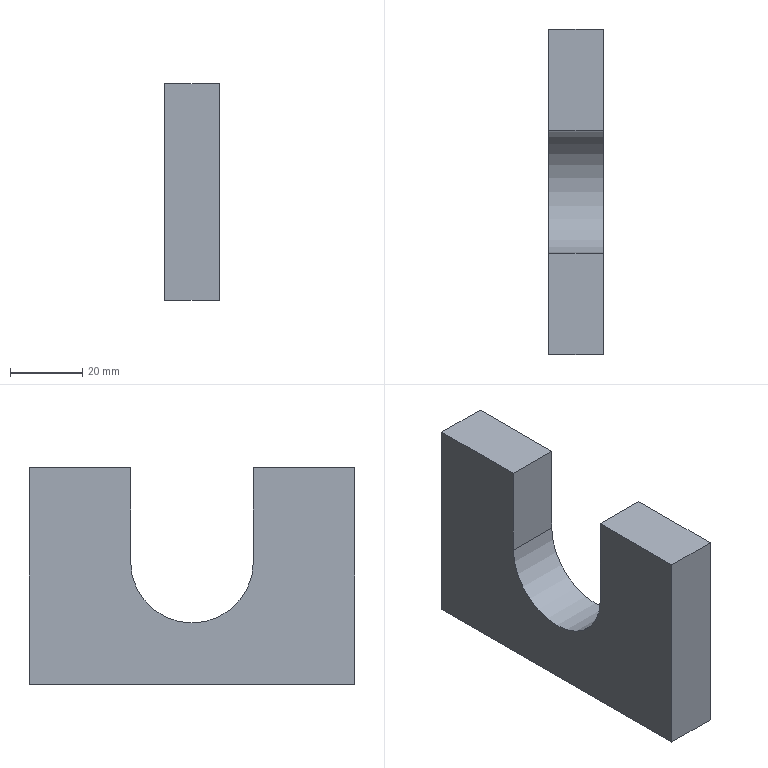Part | STEP file | Tube necking machine_id570_x_t | 1 solid | 10 faces | box 15 x 90 x 60 mm | volume 60931 mm3 | plane 9 | cylinder 1 | commonest cylinder face diameters 34 x1
STEP:
#1=CARTESIAN_POINT('',(0.,0.,0.));
#2=DIRECTION('',(0.,0.,1.));
#3=DIRECTION('',(1.,0.,0.));
#4=AXIS2_PLACEMENT_3D('',#1,#2,#3);
#5=CARTESIAN_POINT('',(305.5,33.,216.));
#6=VERTEX_POINT('',#5);
#7=CARTESIAN_POINT('',(305.5,33.,190.));
#8=VERTEX_POINT('',#7);
#9=CARTESIAN_POINT('',(305.5,33.,252.));
#10=DIRECTION('',(0.,0.,-1.));
#11=VECTOR('',#10,1.);
#12=LINE('',#9,#11);
#13=CARTESIAN_POINT('',(305.5,5.,252.));
#14=DIRECTION('',(-1.,0.,0.));
#15=DIRECTION('',(0.,0.,1.));
#16=AXIS2_PLACEMENT_3D('',#13,#14,#15);
#17=PLANE('',#16);
#18=CARTESIAN_POINT('',(0.,28.));
#19=DIRECTION('',(-1.,0.));
#20=VECTOR('',#19,1.);
#21=LINE('',#18,#20);
#22=(GEOMETRIC_REPRESENTATION_CONTEXT(2)PARAMETRIC_REPRESENTATION_CONTEXT()REPRESENTATION_CONTEXT('',''));
#23=DEFINITIONAL_REPRESENTATION('',(#21),#22);
#24=PCURVE('',#17,#23);
#25=CARTESIAN_POINT('',(320.5,33.,231.));
#26=DIRECTION('',(0.,1.,0.));
#27=DIRECTION('',(0.,0.,1.));
#28=AXIS2_PLACEMENT_3D('',#25,#26,#27);
#29=PLANE('',#28);
#30=CARTESIAN_POINT('',(21.,-15.));
#31=DIRECTION('',(-1.,0.));
#32=VECTOR('',#31,1.);
#33=LINE('',#30,#32);
#34=(GEOMETRIC_REPRESENTATION_CONTEXT(2)PARAMETRIC_REPRESENTATION_CONTEXT()REPRESENTATION_CONTEXT('',''));
#35=DEFINITIONAL_REPRESENTATION('',(#33),#34);
#36=PCURVE('',#29,#35);
#37=SURFACE_CURVE('',#12,(#24,#36),.PCURVE_S1.);
#38=EDGE_CURVE('',#6,#8,#37,.T.);
#39=ORIENTED_EDGE('',*,*,#38,.F.);
#40=CARTESIAN_POINT('',(305.5,5.,216.));
#41=VERTEX_POINT('',#40);
#42=CARTESIAN_POINT('',(305.5,5.,216.));
#43=DIRECTION('',(0.,1.,0.));
#44=VECTOR('',#43,1.);
#45=LINE('',#42,#44);
#46=CARTESIAN_POINT('',(-36.,0.));
#47=DIRECTION('',(0.,1.));
#48=VECTOR('',#47,1.);
#49=LINE('',#46,#48);
#50=(GEOMETRIC_REPRESENTATION_CONTEXT(2)PARAMETRIC_REPRESENTATION_CONTEXT()REPRESENTATION_CONTEXT('',''));
#51=DEFINITIONAL_REPRESENTATION('',(#49),#50);
#52=PCURVE('',#17,#51);
#53=CARTESIAN_POINT('',(8.,0.,216.));
#54=DIRECTION('',(0.,0.,1.));
#55=DIRECTION('',(1.,0.,0.));
#56=AXIS2_PLACEMENT_3D('',#53,#54,#55);
#57=PLANE('',#56);
#58=CARTESIAN_POINT('',(297.5,5.));
#59=DIRECTION('',(0.,1.));
#60=VECTOR('',#59,1.);
#61=LINE('',#58,#60);
#62=(GEOMETRIC_REPRESENTATION_CONTEXT(2)PARAMETRIC_REPRESENTATION_CONTEXT()REPRESENTATION_CONTEXT('',''));
#63=DEFINITIONAL_REPRESENTATION('',(#61),#62);
#64=PCURVE('',#57,#63);
#65=SURFACE_CURVE('',#45,(#52,#64),.PCURVE_S1.);
#66=EDGE_CURVE('',#41,#6,#65,.T.);
#67=ORIENTED_EDGE('',*,*,#66,.F.);
#68=CARTESIAN_POINT('',(305.5,5.,156.));
#69=VERTEX_POINT('',#68);
#70=CARTESIAN_POINT('',(305.5,5.,252.));
#71=DIRECTION('',(0.,0.,-1.));
#72=VECTOR('',#71,1.);
#73=LINE('',#70,#72);
#74=CARTESIAN_POINT('',(0.,0.));
#75=DIRECTION('',(-1.,0.));
#76=VECTOR('',#75,1.);
#77=LINE('',#74,#76);
#78=(GEOMETRIC_REPRESENTATION_CONTEXT(2)PARAMETRIC_REPRESENTATION_CONTEXT()REPRESENTATION_CONTEXT('',''));
#79=DEFINITIONAL_REPRESENTATION('',(#77),#78);
#80=PCURVE('',#17,#79);
#81=CARTESIAN_POINT('',(235.5,5.,252.));
#82=DIRECTION('',(0.,1.,0.));
#83=DIRECTION('',(0.,0.,1.));
#84=AXIS2_PLACEMENT_3D('',#81,#82,#83);
#85=PLANE('',#84);
#86=CARTESIAN_POINT('',(0.,70.));
#87=DIRECTION('',(-1.,0.));
#88=VECTOR('',#87,1.);
#89=LINE('',#86,#88);
#90=(GEOMETRIC_REPRESENTATION_CONTEXT(2)PARAMETRIC_REPRESENTATION_CONTEXT()REPRESENTATION_CONTEXT('',''));
#91=DEFINITIONAL_REPRESENTATION('',(#89),#90);
#92=PCURVE('',#85,#91);
#93=SURFACE_CURVE('',#73,(#80,#92),.PCURVE_S1.);
#94=EDGE_CURVE('',#41,#69,#93,.T.);
#95=ORIENTED_EDGE('',*,*,#94,.T.);
#96=CARTESIAN_POINT('',(305.5,95.,156.));
#97=VERTEX_POINT('',#96);
#98=CARTESIAN_POINT('',(305.5,5.,156.));
#99=DIRECTION('',(0.,1.,0.));
#100=VECTOR('',#99,1.);
#101=LINE('',#98,#100);
#102=CARTESIAN_POINT('',(-96.,0.));
#103=DIRECTION('',(0.,1.));
#104=VECTOR('',#103,1.);
#105=LINE('',#102,#104);
#106=(GEOMETRIC_REPRESENTATION_CONTEXT(2)PARAMETRIC_REPRESENTATION_CONTEXT()REPRESENTATION_CONTEXT('',''));
#107=DEFINITIONAL_REPRESENTATION('',(#105),#106);
#108=PCURVE('',#17,#107);
#109=CARTESIAN_POINT('',(8.,0.,156.));
#110=DIRECTION('',(0.,0.,1.));
#111=DIRECTION('',(1.,0.,0.));
#112=AXIS2_PLACEMENT_3D('',#109,#110,#111);
#113=PLANE('',#112);
#114=CARTESIAN_POINT('',(297.5,5.));
#115=DIRECTION('',(0.,1.));
#116=VECTOR('',#115,1.);
#117=LINE('',#114,#116);
#118=(GEOMETRIC_REPRESENTATION_CONTEXT(2)PARAMETRIC_REPRESENTATION_CONTEXT()REPRESENTATION_CONTEXT('',''));
#119=DEFINITIONAL_REPRESENTATION('',(#117),#118);
#120=PCURVE('',#113,#119);
#121=SURFACE_CURVE('',#101,(#108,#120),.PCURVE_S1.);
#122=EDGE_CURVE('',#69,#97,#121,.T.);
#123=ORIENTED_EDGE('',*,*,#122,.T.);
#124=CARTESIAN_POINT('',(305.5,95.,216.));
#125=VERTEX_POINT('',#124);
#126=CARTESIAN_POINT('',(305.5,95.,252.));
#127=DIRECTION('',(0.,0.,-1.));
#128=VECTOR('',#127,1.);
#129=LINE('',#126,#128);
#130=CARTESIAN_POINT('',(0.,90.));
#131=DIRECTION('',(-1.,0.));
#132=VECTOR('',#131,1.);
#133=LINE('',#130,#132);
#134=(GEOMETRIC_REPRESENTATION_CONTEXT(2)PARAMETRIC_REPRESENTATION_CONTEXT()REPRESENTATION_CONTEXT('',''));
#135=DEFINITIONAL_REPRESENTATION('',(#133),#134);
#136=PCURVE('',#17,#135);
#137=CARTESIAN_POINT('',(305.5,95.,252.));
#138=DIRECTION('',(0.,-1.,0.));
#139=DIRECTION('',(0.,0.,-1.));
#140=AXIS2_PLACEMENT_3D('',#137,#138,#139);
#141=PLANE('',#140);
#142=CARTESIAN_POINT('',(0.,0.));
#143=DIRECTION('',(1.,0.));
#144=VECTOR('',#143,1.);
#145=LINE('',#142,#144);
#146=(GEOMETRIC_REPRESENTATION_CONTEXT(2)PARAMETRIC_REPRESENTATION_CONTEXT()REPRESENTATION_CONTEXT('',''));
#147=DEFINITIONAL_REPRESENTATION('',(#145),#146);
#148=PCURVE('',#141,#147);
#149=SURFACE_CURVE('',#129,(#136,#148),.PCURVE_S1.);
#150=EDGE_CURVE('',#125,#97,#149,.T.);
#151=ORIENTED_EDGE('',*,*,#150,.F.);
#152=CARTESIAN_POINT('',(305.5,67.,216.));
#153=VERTEX_POINT('',#152);
#154=CARTESIAN_POINT('',(305.5,5.,216.));
#155=DIRECTION('',(0.,1.,0.));
#156=VECTOR('',#155,1.);
#157=LINE('',#154,#156);
#158=CARTESIAN_POINT('',(-36.,0.));
#159=DIRECTION('',(0.,1.));
#160=VECTOR('',#159,1.);
#161=LINE('',#158,#160);
#162=(GEOMETRIC_REPRESENTATION_CONTEXT(2)PARAMETRIC_REPRESENTATION_CONTEXT()REPRESENTATION_CONTEXT('',''));
#163=DEFINITIONAL_REPRESENTATION('',(#161),#162);
#164=PCURVE('',#17,#163);
#165=CARTESIAN_POINT('',(8.,0.,216.));
#166=DIRECTION('',(0.,0.,1.));
#167=DIRECTION('',(1.,0.,0.));
#168=AXIS2_PLACEMENT_3D('',#165,#166,#167);
#169=PLANE('',#168);
#170=CARTESIAN_POINT('',(297.5,5.));
#171=DIRECTION('',(0.,1.));
#172=VECTOR('',#171,1.);
#173=LINE('',#170,#172);
#174=(GEOMETRIC_REPRESENTATION_CONTEXT(2)PARAMETRIC_REPRESENTATION_CONTEXT()REPRESENTATION_CONTEXT('',''));
#175=DEFINITIONAL_REPRESENTATION('',(#173),#174);
#176=PCURVE('',#169,#175);
#177=SURFACE_CURVE('',#157,(#164,#176),.PCURVE_S1.);
#178=EDGE_CURVE('',#153,#125,#177,.T.);
#179=ORIENTED_EDGE('',*,*,#178,.F.);
#180=CARTESIAN_POINT('',(305.5,67.,190.));
#181=VERTEX_POINT('',#180);
#182=CARTESIAN_POINT('',(305.5,67.,252.));
#183=DIRECTION('',(0.,0.,1.));
#184=VECTOR('',#183,1.);
#185=LINE('',#182,#184);
#186=CARTESIAN_POINT('',(0.,62.));
#187=DIRECTION('',(1.,0.));
#188=VECTOR('',#187,1.);
#189=LINE('',#186,#188);
#190=(GEOMETRIC_REPRESENTATION_CONTEXT(2)PARAMETRIC_REPRESENTATION_CONTEXT()REPRESENTATION_CONTEXT('',''));
#191=DEFINITIONAL_REPRESENTATION('',(#189),#190);
#192=PCURVE('',#17,#191);
#193=CARTESIAN_POINT('',(320.5,67.,190.));
#194=DIRECTION('',(0.,-1.,0.));
#195=DIRECTION('',(0.,0.,-1.));
#196=AXIS2_PLACEMENT_3D('',#193,#194,#195);
#197=PLANE('',#196);
#198=CARTESIAN_POINT('',(-62.,-15.));
#199=DIRECTION('',(-1.,0.));
#200=VECTOR('',#199,1.);
#201=LINE('',#198,#200);
#202=(GEOMETRIC_REPRESENTATION_CONTEXT(2)PARAMETRIC_REPRESENTATION_CONTEXT()REPRESENTATION_CONTEXT('',''));
#203=DEFINITIONAL_REPRESENTATION('',(#201),#202);
#204=PCURVE('',#197,#203);
#205=SURFACE_CURVE('',#185,(#192,#204),.PCURVE_S1.);
#206=EDGE_CURVE('',#181,#153,#205,.T.);
#207=ORIENTED_EDGE('',*,*,#206,.F.);
#208=CARTESIAN_POINT('',(305.5,50.,190.));
#209=DIRECTION('',(1.,0.,0.));
#210=DIRECTION('',(0.,0.,1.));
#211=AXIS2_PLACEMENT_3D('',#208,#209,#210);
#212=CIRCLE('',#211,17.);
#213=CARTESIAN_POINT('',(-45.,45.));
#214=CARTESIAN_POINT('',(-45.,15.555));
#215=CARTESIAN_POINT('',(-70.5,30.278));
#216=CARTESIAN_POINT('',(-96.,45.));
#217=CARTESIAN_POINT('',(-70.5,59.722));
#218=CARTESIAN_POINT('',(-45.,74.445));
#219=CARTESIAN_POINT('',(-45.,45.));
#220=(BOUNDED_CURVE()B_SPLINE_CURVE(2,(#213,#214,#215,#216,#217,#218,#219),.UNSPECIFIED.,.T.,.F.)B_SPLINE_CURVE_WITH_KNOTS((1,2,2,2,2,1),(-2.094,0.,2.094,4.189,6.283,8.378),.UNSPECIFIED.)CURVE()GEOMETRIC_REPRESENTATION_ITEM()RATIONAL_B_SPLINE_CURVE((1.,0.5,1.,0.5,1.,0.5,1.))REPRESENTATION_ITEM(''));
#221=(GEOMETRIC_REPRESENTATION_CONTEXT(2)PARAMETRIC_REPRESENTATION_CONTEXT()REPRESENTATION_CONTEXT('',''));
#222=DEFINITIONAL_REPRESENTATION('',(#220),#221);
#223=PCURVE('',#17,#222);
#224=CARTESIAN_POINT('',(290.5,50.,190.));
#225=DIRECTION('',(1.,0.,0.));
#226=DIRECTION('',(0.,0.,-1.));
#227=AXIS2_PLACEMENT_3D('',#224,#225,#226);
#228=CYLINDRICAL_SURFACE('',#227,17.);
#229=CARTESIAN_POINT('',(3.142,15.));
#230=DIRECTION('',(1.,0.));
#231=VECTOR('',#230,1.);
#232=LINE('',#229,#231);
#233=(GEOMETRIC_REPRESENTATION_CONTEXT(2)PARAMETRIC_REPRESENTATION_CONTEXT()REPRESENTATION_CONTEXT('',''));
#234=DEFINITIONAL_REPRESENTATION('',(#232),#233);
#235=PCURVE('',#228,#234);
#236=SURFACE_CURVE('',#212,(#223,#235),.PCURVE_S1.);
#237=EDGE_CURVE('',#8,#181,#236,.T.);
#238=ORIENTED_EDGE('',*,*,#237,.F.);
#239=EDGE_LOOP('',(#39,#67,#95,#123,#151,#179,#207,#238));
#240=FACE_BOUND('',#239,.T.);
#241=ADVANCED_FACE('',(#240),#17,.F.);
#242=ORIENTED_EDGE('',*,*,#66,.T.);
#243=CARTESIAN_POINT('',(290.5,33.,216.));
#244=VERTEX_POINT('',#243);
#245=CARTESIAN_POINT('',(8.,33.,216.));
#246=DIRECTION('',(-1.,0.,0.));
#247=VECTOR('',#246,1.);
#248=LINE('',#245,#247);
#249=CARTESIAN_POINT('',(0.,33.));
#250=DIRECTION('',(-1.,0.));
#251=VECTOR('',#250,1.);
#252=LINE('',#249,#251);
#253=(GEOMETRIC_REPRESENTATION_CONTEXT(2)PARAMETRIC_REPRESENTATION_CONTEXT()REPRESENTATION_CONTEXT('',''));
#254=DEFINITIONAL_REPRESENTATION('',(#252),#253);
#255=PCURVE('',#57,#254);
#256=CARTESIAN_POINT('',(-15.,-312.5));
#257=DIRECTION('',(0.,-1.));
#258=VECTOR('',#257,1.);
#259=LINE('',#256,#258);
#260=(GEOMETRIC_REPRESENTATION_CONTEXT(2)PARAMETRIC_REPRESENTATION_CONTEXT()REPRESENTATION_CONTEXT('',''));
#261=DEFINITIONAL_REPRESENTATION('',(#259),#260);
#262=PCURVE('',#29,#261);
#263=SURFACE_CURVE('',#248,(#255,#262),.PCURVE_S1.);
#264=EDGE_CURVE('',#6,#244,#263,.T.);
#265=ORIENTED_EDGE('',*,*,#264,.T.);
#266=CARTESIAN_POINT('',(290.5,5.,216.));
#267=VERTEX_POINT('',#266);
#268=CARTESIAN_POINT('',(290.5,0.,216.));
#269=DIRECTION('',(0.,1.,0.));
#270=VECTOR('',#269,1.);
#271=LINE('',#268,#270);
#272=CARTESIAN_POINT('',(282.5,0.));
#273=DIRECTION('',(0.,1.));
#274=VECTOR('',#273,1.);
#275=LINE('',#272,#274);
#276=(GEOMETRIC_REPRESENTATION_CONTEXT(2)PARAMETRIC_REPRESENTATION_CONTEXT()REPRESENTATION_CONTEXT('',''));
#277=DEFINITIONAL_REPRESENTATION('',(#275),#276);
#278=PCURVE('',#57,#277);
#279=CARTESIAN_POINT('',(290.5,20.,332.));
#280=DIRECTION('',(-1.,0.,0.));
#281=DIRECTION('',(0.,0.,1.));
#282=AXIS2_PLACEMENT_3D('',#279,#280,#281);
#283=PLANE('',#282);
#284=CARTESIAN_POINT('',(-116.,-20.));
#285=DIRECTION('',(0.,1.));
#286=VECTOR('',#285,1.);
#287=LINE('',#284,#286);
#288=(GEOMETRIC_REPRESENTATION_CONTEXT(2)PARAMETRIC_REPRESENTATION_CONTEXT()REPRESENTATION_CONTEXT('',''));
#289=DEFINITIONAL_REPRESENTATION('',(#287),#288);
#290=PCURVE('',#283,#289);
#291=SURFACE_CURVE('',#271,(#278,#290),.PCURVE_S1.);
#292=EDGE_CURVE('',#267,#244,#291,.T.);
#293=ORIENTED_EDGE('',*,*,#292,.F.);
#294=CARTESIAN_POINT('',(235.5,5.,216.));
#295=DIRECTION('',(1.,0.,0.));
#296=VECTOR('',#295,1.);
#297=LINE('',#294,#296);
#298=CARTESIAN_POINT('',(227.5,5.));
#299=DIRECTION('',(1.,0.));
#300=VECTOR('',#299,1.);
#301=LINE('',#298,#300);
#302=(GEOMETRIC_REPRESENTATION_CONTEXT(2)PARAMETRIC_REPRESENTATION_CONTEXT()REPRESENTATION_CONTEXT('',''));
#303=DEFINITIONAL_REPRESENTATION('',(#301),#302);
#304=PCURVE('',#57,#303);
#305=CARTESIAN_POINT('',(-36.,0.));
#306=DIRECTION('',(0.,1.));
#307=VECTOR('',#306,1.);
#308=LINE('',#305,#307);
#309=(GEOMETRIC_REPRESENTATION_CONTEXT(2)PARAMETRIC_REPRESENTATION_CONTEXT()REPRESENTATION_CONTEXT('',''));
#310=DEFINITIONAL_REPRESENTATION('',(#308),#309);
#311=PCURVE('',#85,#310);
#312=SURFACE_CURVE('',#297,(#304,#311),.PCURVE_S1.);
#313=EDGE_CURVE('',#267,#41,#312,.T.);
#314=ORIENTED_EDGE('',*,*,#313,.T.);
#315=EDGE_LOOP('',(#242,#265,#293,#314));
#316=FACE_BOUND('',#315,.T.);
#317=ADVANCED_FACE('',(#316),#57,.T.);
#318=CARTESIAN_POINT('',(290.5,67.,216.));
#319=VERTEX_POINT('',#318);
#320=CARTESIAN_POINT('',(290.5,95.,216.));
#321=VERTEX_POINT('',#320);
#322=CARTESIAN_POINT('',(290.5,0.,216.));
#323=DIRECTION('',(0.,1.,0.));
#324=VECTOR('',#323,1.);
#325=LINE('',#322,#324);
#326=CARTESIAN_POINT('',(282.5,0.));
#327=DIRECTION('',(0.,1.));
#328=VECTOR('',#327,1.);
#329=LINE('',#326,#328);
#330=(GEOMETRIC_REPRESENTATION_CONTEXT(2)PARAMETRIC_REPRESENTATION_CONTEXT()REPRESENTATION_CONTEXT('',''));
#331=DEFINITIONAL_REPRESENTATION('',(#329),#330);
#332=PCURVE('',#169,#331);
#333=CARTESIAN_POINT('',(-116.,-20.));
#334=DIRECTION('',(0.,1.));
#335=VECTOR('',#334,1.);
#336=LINE('',#333,#335);
#337=(GEOMETRIC_REPRESENTATION_CONTEXT(2)PARAMETRIC_REPRESENTATION_CONTEXT()REPRESENTATION_CONTEXT('',''));
#338=DEFINITIONAL_REPRESENTATION('',(#336),#337);
#339=PCURVE('',#283,#338);
#340=SURFACE_CURVE('',#325,(#332,#339),.PCURVE_S1.);
#341=EDGE_CURVE('',#319,#321,#340,.T.);
#342=ORIENTED_EDGE('',*,*,#341,.F.);
#343=CARTESIAN_POINT('',(8.,67.,216.));
#344=DIRECTION('',(1.,0.,0.));
#345=VECTOR('',#344,1.);
#346=LINE('',#343,#345);
#347=CARTESIAN_POINT('',(0.,67.));
#348=DIRECTION('',(1.,0.));
#349=VECTOR('',#348,1.);
#350=LINE('',#347,#349);
#351=(GEOMETRIC_REPRESENTATION_CONTEXT(2)PARAMETRIC_REPRESENTATION_CONTEXT()REPRESENTATION_CONTEXT('',''));
#352=DEFINITIONAL_REPRESENTATION('',(#350),#351);
#353=PCURVE('',#169,#352);
#354=CARTESIAN_POINT('',(-26.,-312.5));
#355=DIRECTION('',(0.,1.));
#356=VECTOR('',#355,1.);
#357=LINE('',#354,#356);
#358=(GEOMETRIC_REPRESENTATION_CONTEXT(2)PARAMETRIC_REPRESENTATION_CONTEXT()REPRESENTATION_CONTEXT('',''));
#359=DEFINITIONAL_REPRESENTATION('',(#357),#358);
#360=PCURVE('',#197,#359);
#361=SURFACE_CURVE('',#346,(#353,#360),.PCURVE_S1.);
#362=EDGE_CURVE('',#319,#153,#361,.T.);
#363=ORIENTED_EDGE('',*,*,#362,.T.);
#364=ORIENTED_EDGE('',*,*,#178,.T.);
#365=CARTESIAN_POINT('',(305.5,95.,216.));
#366=DIRECTION('',(-1.,0.,0.));
#367=VECTOR('',#366,1.);
#368=LINE('',#365,#367);
#369=CARTESIAN_POINT('',(297.5,95.));
#370=DIRECTION('',(-1.,0.));
#371=VECTOR('',#370,1.);
#372=LINE('',#369,#371);
#373=(GEOMETRIC_REPRESENTATION_CONTEXT(2)PARAMETRIC_REPRESENTATION_CONTEXT()REPRESENTATION_CONTEXT('',''));
#374=DEFINITIONAL_REPRESENTATION('',(#372),#373);
#375=PCURVE('',#169,#374);
#376=CARTESIAN_POINT('',(36.,0.));
#377=DIRECTION('',(0.,-1.));
#378=VECTOR('',#377,1.);
#379=LINE('',#376,#378);
#380=(GEOMETRIC_REPRESENTATION_CONTEXT(2)PARAMETRIC_REPRESENTATION_CONTEXT()REPRESENTATION_CONTEXT('',''));
#381=DEFINITIONAL_REPRESENTATION('',(#379),#380);
#382=PCURVE('',#141,#381);
#383=SURFACE_CURVE('',#368,(#375,#382),.PCURVE_S1.);
#384=EDGE_CURVE('',#125,#321,#383,.T.);
#385=ORIENTED_EDGE('',*,*,#384,.T.);
#386=EDGE_LOOP('',(#342,#363,#364,#385));
#387=FACE_BOUND('',#386,.T.);
#388=ADVANCED_FACE('',(#387),#169,.T.);
#389=ORIENTED_EDGE('',*,*,#292,.T.);
#390=CARTESIAN_POINT('',(290.5,33.,190.));
#391=VERTEX_POINT('',#390);
#392=CARTESIAN_POINT('',(290.5,33.,332.));
#393=DIRECTION('',(0.,0.,-1.));
#394=VECTOR('',#393,1.);
#395=LINE('',#392,#394);
#396=CARTESIAN_POINT('',(0.,13.));
#397=DIRECTION('',(-1.,0.));
#398=VECTOR('',#397,1.);
#399=LINE('',#396,#398);
#400=(GEOMETRIC_REPRESENTATION_CONTEXT(2)PARAMETRIC_REPRESENTATION_CONTEXT()REPRESENTATION_CONTEXT('',''));
#401=DEFINITIONAL_REPRESENTATION('',(#399),#400);
#402=PCURVE('',#283,#401);
#403=CARTESIAN_POINT('',(101.,-30.));
#404=DIRECTION('',(-1.,0.));
#405=VECTOR('',#404,1.);
#406=LINE('',#403,#405);
#407=(GEOMETRIC_REPRESENTATION_CONTEXT(2)PARAMETRIC_REPRESENTATION_CONTEXT()REPRESENTATION_CONTEXT('',''));
#408=DEFINITIONAL_REPRESENTATION('',(#406),#407);
#409=PCURVE('',#29,#408);
#410=SURFACE_CURVE('',#395,(#402,#409),.PCURVE_S1.);
#411=EDGE_CURVE('',#244,#391,#410,.T.);
#412=ORIENTED_EDGE('',*,*,#411,.T.);
#413=CARTESIAN_POINT('',(290.5,67.,190.));
#414=VERTEX_POINT('',#413);
#415=CARTESIAN_POINT('',(290.5,50.,190.));
#416=DIRECTION('',(1.,0.,0.));
#417=DIRECTION('',(0.,0.,1.));
#418=AXIS2_PLACEMENT_3D('',#415,#416,#417);
#419=CIRCLE('',#418,17.);
#420=CARTESIAN_POINT('',(-125.,30.));
#421=CARTESIAN_POINT('',(-125.,0.5551));
#422=CARTESIAN_POINT('',(-150.5,15.278));
#423=CARTESIAN_POINT('',(-176.,30.));
#424=CARTESIAN_POINT('',(-150.5,44.722));
#425=CARTESIAN_POINT('',(-125.,59.445));
#426=CARTESIAN_POINT('',(-125.,30.));
#427=(BOUNDED_CURVE()B_SPLINE_CURVE(2,(#420,#421,#422,#423,#424,#425,#426),.UNSPECIFIED.,.T.,.F.)B_SPLINE_CURVE_WITH_KNOTS((1,2,2,2,2,1),(-2.094,0.,2.094,4.189,6.283,8.378),.UNSPECIFIED.)CURVE()GEOMETRIC_REPRESENTATION_ITEM()RATIONAL_B_SPLINE_CURVE((1.,0.5,1.,0.5,1.,0.5,1.))REPRESENTATION_ITEM(''));
#428=(GEOMETRIC_REPRESENTATION_CONTEXT(2)PARAMETRIC_REPRESENTATION_CONTEXT()REPRESENTATION_CONTEXT('',''));
#429=DEFINITIONAL_REPRESENTATION('',(#427),#428);
#430=PCURVE('',#283,#429);
#431=CARTESIAN_POINT('',(3.142,0.));
#432=DIRECTION('',(1.,0.));
#433=VECTOR('',#432,1.);
#434=LINE('',#431,#433);
#435=(GEOMETRIC_REPRESENTATION_CONTEXT(2)PARAMETRIC_REPRESENTATION_CONTEXT()REPRESENTATION_CONTEXT('',''));
#436=DEFINITIONAL_REPRESENTATION('',(#434),#435);
#437=PCURVE('',#228,#436);
#438=SURFACE_CURVE('',#419,(#430,#437),.PCURVE_S1.);
#439=EDGE_CURVE('',#391,#414,#438,.T.);
#440=ORIENTED_EDGE('',*,*,#439,.T.);
#441=CARTESIAN_POINT('',(290.5,67.,332.));
#442=DIRECTION('',(0.,0.,1.));
#443=VECTOR('',#442,1.);
#444=LINE('',#441,#443);
#445=CARTESIAN_POINT('',(0.,47.));
#446=DIRECTION('',(1.,0.));
#447=VECTOR('',#446,1.);
#448=LINE('',#445,#447);
#449=(GEOMETRIC_REPRESENTATION_CONTEXT(2)PARAMETRIC_REPRESENTATION_CONTEXT()REPRESENTATION_CONTEXT('',''));
#450=DEFINITIONAL_REPRESENTATION('',(#448),#449);
#451=PCURVE('',#283,#450);
#452=CARTESIAN_POINT('',(-142.,-30.));
#453=DIRECTION('',(-1.,0.));
#454=VECTOR('',#453,1.);
#455=LINE('',#452,#454);
#456=(GEOMETRIC_REPRESENTATION_CONTEXT(2)PARAMETRIC_REPRESENTATION_CONTEXT()REPRESENTATION_CONTEXT('',''));
#457=DEFINITIONAL_REPRESENTATION('',(#455),#456);
#458=PCURVE('',#197,#457);
#459=SURFACE_CURVE('',#444,(#451,#458),.PCURVE_S1.);
#460=EDGE_CURVE('',#414,#319,#459,.T.);
#461=ORIENTED_EDGE('',*,*,#460,.T.);
#462=ORIENTED_EDGE('',*,*,#341,.T.);
#463=CARTESIAN_POINT('',(290.5,95.,156.));
#464=VERTEX_POINT('',#463);
#465=CARTESIAN_POINT('',(290.5,95.,252.));
#466=DIRECTION('',(0.,0.,-1.));
#467=VECTOR('',#466,1.);
#468=LINE('',#465,#467);
#469=CARTESIAN_POINT('',(-80.,75.));
#470=DIRECTION('',(-1.,0.));
#471=VECTOR('',#470,1.);
#472=LINE('',#469,#471);
#473=(GEOMETRIC_REPRESENTATION_CONTEXT(2)PARAMETRIC_REPRESENTATION_CONTEXT()REPRESENTATION_CONTEXT('',''));
#474=DEFINITIONAL_REPRESENTATION('',(#472),#473);
#475=PCURVE('',#283,#474);
#476=CARTESIAN_POINT('',(0.,-15.));
#477=DIRECTION('',(1.,0.));
#478=VECTOR('',#477,1.);
#479=LINE('',#476,#478);
#480=(GEOMETRIC_REPRESENTATION_CONTEXT(2)PARAMETRIC_REPRESENTATION_CONTEXT()REPRESENTATION_CONTEXT('',''));
#481=DEFINITIONAL_REPRESENTATION('',(#479),#480);
#482=PCURVE('',#141,#481);
#483=SURFACE_CURVE('',#468,(#475,#482),.PCURVE_S1.);
#484=EDGE_CURVE('',#321,#464,#483,.T.);
#485=ORIENTED_EDGE('',*,*,#484,.T.);
#486=CARTESIAN_POINT('',(290.5,5.,156.));
#487=VERTEX_POINT('',#486);
#488=CARTESIAN_POINT('',(290.5,0.,156.));
#489=DIRECTION('',(0.,1.,0.));
#490=VECTOR('',#489,1.);
#491=LINE('',#488,#490);
#492=CARTESIAN_POINT('',(-176.,-20.));
#493=DIRECTION('',(0.,1.));
#494=VECTOR('',#493,1.);
#495=LINE('',#492,#494);
#496=(GEOMETRIC_REPRESENTATION_CONTEXT(2)PARAMETRIC_REPRESENTATION_CONTEXT()REPRESENTATION_CONTEXT('',''));
#497=DEFINITIONAL_REPRESENTATION('',(#495),#496);
#498=PCURVE('',#283,#497);
#499=CARTESIAN_POINT('',(282.5,0.));
#500=DIRECTION('',(0.,1.));
#501=VECTOR('',#500,1.);
#502=LINE('',#499,#501);
#503=(GEOMETRIC_REPRESENTATION_CONTEXT(2)PARAMETRIC_REPRESENTATION_CONTEXT()REPRESENTATION_CONTEXT('',''));
#504=DEFINITIONAL_REPRESENTATION('',(#502),#503);
#505=PCURVE('',#113,#504);
#506=SURFACE_CURVE('',#491,(#498,#505),.PCURVE_S1.);
#507=EDGE_CURVE('',#487,#464,#506,.T.);
#508=ORIENTED_EDGE('',*,*,#507,.F.);
#509=CARTESIAN_POINT('',(290.5,5.,252.));
#510=DIRECTION('',(0.,0.,1.));
#511=VECTOR('',#510,1.);
#512=LINE('',#509,#511);
#513=CARTESIAN_POINT('',(-80.,-15.));
#514=DIRECTION('',(1.,0.));
#515=VECTOR('',#514,1.);
#516=LINE('',#513,#515);
#517=(GEOMETRIC_REPRESENTATION_CONTEXT(2)PARAMETRIC_REPRESENTATION_CONTEXT()REPRESENTATION_CONTEXT('',''));
#518=DEFINITIONAL_REPRESENTATION('',(#516),#517);
#519=PCURVE('',#283,#518);
#520=CARTESIAN_POINT('',(0.,55.));
#521=DIRECTION('',(1.,0.));
#522=VECTOR('',#521,1.);
#523=LINE('',#520,#522);
#524=(GEOMETRIC_REPRESENTATION_CONTEXT(2)PARAMETRIC_REPRESENTATION_CONTEXT()REPRESENTATION_CONTEXT('',''));
#525=DEFINITIONAL_REPRESENTATION('',(#523),#524);
#526=PCURVE('',#85,#525);
#527=SURFACE_CURVE('',#512,(#519,#526),.PCURVE_S1.);
#528=EDGE_CURVE('',#487,#267,#527,.T.);
#529=ORIENTED_EDGE('',*,*,#528,.T.);
#530=EDGE_LOOP('',(#389,#412,#440,#461,#462,#485,#508,#529));
#531=FACE_BOUND('',#530,.T.);
#532=ADVANCED_FACE('',(#531),#283,.T.);
#533=ORIENTED_EDGE('',*,*,#439,.T.);
#534=CARTESIAN_POINT('',(290.5,67.,190.));
#535=DIRECTION('',(-1.,0.,0.));
#536=VECTOR('',#535,1.);
#537=LINE('',#534,#536);
#538=CARTESIAN_POINT('',(7.854,0.));
#539=DIRECTION('',(0.,-1.));
#540=VECTOR('',#539,1.);
#541=LINE('',#538,#540);
#542=(GEOMETRIC_REPRESENTATION_CONTEXT(2)PARAMETRIC_REPRESENTATION_CONTEXT()REPRESENTATION_CONTEXT('',''));
#543=DEFINITIONAL_REPRESENTATION('',(#541),#542);
#544=PCURVE('',#228,#543);
#545=CARTESIAN_POINT('',(0.,-30.));
#546=DIRECTION('',(0.,-1.));
#547=VECTOR('',#546,1.);
#548=LINE('',#545,#547);
#549=(GEOMETRIC_REPRESENTATION_CONTEXT(2)PARAMETRIC_REPRESENTATION_CONTEXT()REPRESENTATION_CONTEXT('',''));
#550=DEFINITIONAL_REPRESENTATION('',(#548),#549);
#551=PCURVE('',#197,#550);
#552=SURFACE_CURVE('',#537,(#544,#551),.PCURVE_S1.);
#553=EDGE_CURVE('',#181,#414,#552,.T.);
#554=ORIENTED_EDGE('',*,*,#553,.F.);
#555=ORIENTED_EDGE('',*,*,#237,.F.);
#556=CARTESIAN_POINT('',(320.5,33.,190.));
#557=DIRECTION('',(-1.,0.,0.));
#558=VECTOR('',#557,1.);
#559=LINE('',#556,#558);
#560=CARTESIAN_POINT('',(4.712,30.));
#561=DIRECTION('',(0.,-1.));
#562=VECTOR('',#561,1.);
#563=LINE('',#560,#562);
#564=(GEOMETRIC_REPRESENTATION_CONTEXT(2)PARAMETRIC_REPRESENTATION_CONTEXT()REPRESENTATION_CONTEXT('',''));
#565=DEFINITIONAL_REPRESENTATION('',(#563),#564);
#566=PCURVE('',#228,#565);
#567=CARTESIAN_POINT('',(-41.,0.));
#568=DIRECTION('',(0.,-1.));
#569=VECTOR('',#568,1.);
#570=LINE('',#567,#569);
#571=(GEOMETRIC_REPRESENTATION_CONTEXT(2)PARAMETRIC_REPRESENTATION_CONTEXT()REPRESENTATION_CONTEXT('',''));
#572=DEFINITIONAL_REPRESENTATION('',(#570),#571);
#573=PCURVE('',#29,#572);
#574=SURFACE_CURVE('',#559,(#566,#573),.PCURVE_S1.);
#575=EDGE_CURVE('',#8,#391,#574,.T.);
#576=ORIENTED_EDGE('',*,*,#575,.T.);
#577=EDGE_LOOP('',(#533,#554,#555,#576));
#578=FACE_BOUND('',#577,.F.);
#579=ADVANCED_FACE('',(#578),#228,.F.);
#580=ORIENTED_EDGE('',*,*,#507,.T.);
#581=CARTESIAN_POINT('',(305.5,95.,156.));
#582=DIRECTION('',(-1.,0.,0.));
#583=VECTOR('',#582,1.);
#584=LINE('',#581,#583);
#585=CARTESIAN_POINT('',(297.5,95.));
#586=DIRECTION('',(-1.,0.));
#587=VECTOR('',#586,1.);
#588=LINE('',#585,#587);
#589=(GEOMETRIC_REPRESENTATION_CONTEXT(2)PARAMETRIC_REPRESENTATION_CONTEXT()REPRESENTATION_CONTEXT('',''));
#590=DEFINITIONAL_REPRESENTATION('',(#588),#589);
#591=PCURVE('',#113,#590);
#592=CARTESIAN_POINT('',(96.,0.));
#593=DIRECTION('',(0.,-1.));
#594=VECTOR('',#593,1.);
#595=LINE('',#592,#594);
#596=(GEOMETRIC_REPRESENTATION_CONTEXT(2)PARAMETRIC_REPRESENTATION_CONTEXT()REPRESENTATION_CONTEXT('',''));
#597=DEFINITIONAL_REPRESENTATION('',(#595),#596);
#598=PCURVE('',#141,#597);
#599=SURFACE_CURVE('',#584,(#591,#598),.PCURVE_S1.);
#600=EDGE_CURVE('',#97,#464,#599,.T.);
#601=ORIENTED_EDGE('',*,*,#600,.F.);
#602=ORIENTED_EDGE('',*,*,#122,.F.);
#603=CARTESIAN_POINT('',(235.5,5.,156.));
#604=DIRECTION('',(1.,0.,0.));
#605=VECTOR('',#604,1.);
#606=LINE('',#603,#605);
#607=CARTESIAN_POINT('',(227.5,5.));
#608=DIRECTION('',(1.,0.));
#609=VECTOR('',#608,1.);
#610=LINE('',#607,#609);
#611=(GEOMETRIC_REPRESENTATION_CONTEXT(2)PARAMETRIC_REPRESENTATION_CONTEXT()REPRESENTATION_CONTEXT('',''));
#612=DEFINITIONAL_REPRESENTATION('',(#610),#611);
#613=PCURVE('',#113,#612);
#614=CARTESIAN_POINT('',(-96.,0.));
#615=DIRECTION('',(0.,1.));
#616=VECTOR('',#615,1.);
#617=LINE('',#614,#616);
#618=(GEOMETRIC_REPRESENTATION_CONTEXT(2)PARAMETRIC_REPRESENTATION_CONTEXT()REPRESENTATION_CONTEXT('',''));
#619=DEFINITIONAL_REPRESENTATION('',(#617),#618);
#620=PCURVE('',#85,#619);
#621=SURFACE_CURVE('',#606,(#613,#620),.PCURVE_S1.);
#622=EDGE_CURVE('',#487,#69,#621,.T.);
#623=ORIENTED_EDGE('',*,*,#622,.F.);
#624=EDGE_LOOP('',(#580,#601,#602,#623));
#625=FACE_BOUND('',#624,.T.);
#626=ADVANCED_FACE('',(#625),#113,.F.);
#627=ORIENTED_EDGE('',*,*,#528,.F.);
#628=ORIENTED_EDGE('',*,*,#622,.T.);
#629=ORIENTED_EDGE('',*,*,#94,.F.);
#630=ORIENTED_EDGE('',*,*,#313,.F.);
#631=EDGE_LOOP('',(#627,#628,#629,#630));
#632=FACE_BOUND('',#631,.T.);
#633=ADVANCED_FACE('',(#632),#85,.F.);
#634=ORIENTED_EDGE('',*,*,#484,.F.);
#635=ORIENTED_EDGE('',*,*,#384,.F.);
#636=ORIENTED_EDGE('',*,*,#150,.T.);
#637=ORIENTED_EDGE('',*,*,#600,.T.);
#638=EDGE_LOOP('',(#634,#635,#636,#637));
#639=FACE_BOUND('',#638,.T.);
#640=ADVANCED_FACE('',(#639),#141,.F.);
#641=ORIENTED_EDGE('',*,*,#206,.T.);
#642=ORIENTED_EDGE('',*,*,#362,.F.);
#643=ORIENTED_EDGE('',*,*,#460,.F.);
#644=ORIENTED_EDGE('',*,*,#553,.F.);
#645=EDGE_LOOP('',(#641,#642,#643,#644));
#646=FACE_BOUND('',#645,.T.);
#647=ADVANCED_FACE('',(#646),#197,.T.);
#648=ORIENTED_EDGE('',*,*,#38,.T.);
#649=ORIENTED_EDGE('',*,*,#575,.T.);
#650=ORIENTED_EDGE('',*,*,#411,.F.);
#651=ORIENTED_EDGE('',*,*,#264,.F.);
#652=EDGE_LOOP('',(#648,#649,#650,#651));
#653=FACE_BOUND('',#652,.T.);
#654=ADVANCED_FACE('',(#653),#29,.T.);
#655=CLOSED_SHELL('',(#241,#317,#388,#532,#579,#626,#633,#640,#647,#654));
#656=MANIFOLD_SOLID_BREP('',#655);
#657=(LENGTH_UNIT()NAMED_UNIT(*)SI_UNIT(.MILLI.,.METRE.));
#658=UNCERTAINTY_MEASURE_WITH_UNIT(LENGTH_MEASURE(0.0000001),#657,'','');
#659=(NAMED_UNIT(*)PLANE_ANGLE_UNIT()SI_UNIT($,.RADIAN.));
#660=(NAMED_UNIT(*)SI_UNIT($,.STERADIAN.)SOLID_ANGLE_UNIT());
#661=(GEOMETRIC_REPRESENTATION_CONTEXT(3)GLOBAL_UNCERTAINTY_ASSIGNED_CONTEXT((#658))GLOBAL_UNIT_ASSIGNED_CONTEXT((#657,#659,#660))REPRESENTATION_CONTEXT('',''));
#662=ADVANCED_BREP_SHAPE_REPRESENTATION('',(#4,#656),#661);